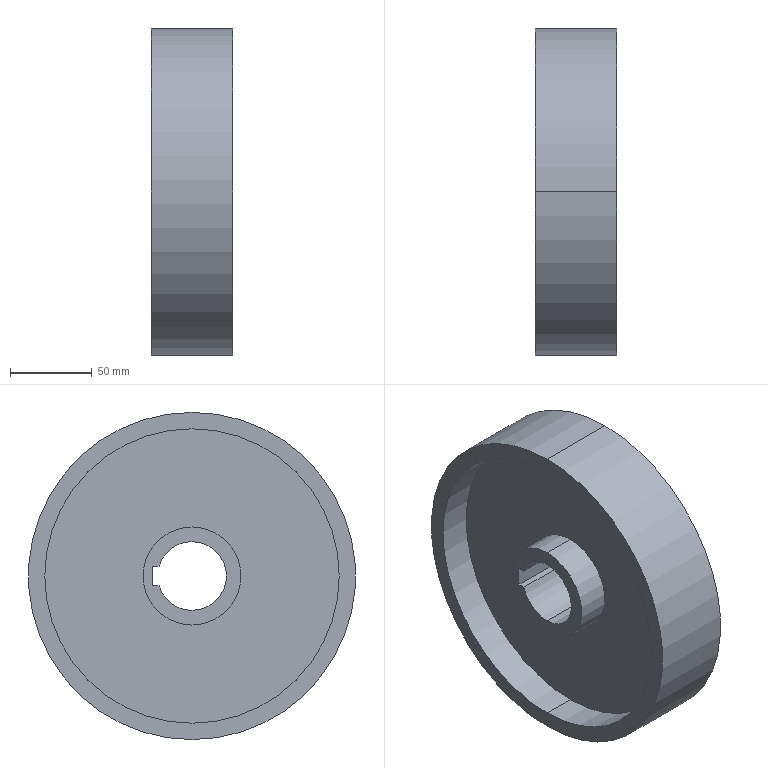Part | SolidWorks | features ICE 1, Revolution 1 | 1 solid | 22 faces | box 50 x 200 x 200 mm | volume 594592 mm3 | cylinder 13 | plane 9 | commonest cylinder face diameters 60 x4 180 x4 42 x3 200 x2
STEP:
#1=CARTESIAN_POINT('',(25.,0.,-21.));
#2=VERTEX_POINT('',#1);
#3=CARTESIAN_POINT('',(25.,0.,21.));
#4=VERTEX_POINT('',#3);
#5=CARTESIAN_POINT('',(25.,0.,0.));
#6=DIRECTION('',(-1.,0.,0.));
#7=DIRECTION('',(0.,0.,1.));
#8=AXIS2_PLACEMENT_3D('',#5,#6,#7);
#9=CIRCLE('',#8,21.);
#10=EDGE_CURVE('',#2,#4,#9,.T.);
#11=ORIENTED_EDGE('',*,*,#10,.F.);
#12=CARTESIAN_POINT('',(-25.,0.,-21.));
#13=VERTEX_POINT('',#12);
#14=CARTESIAN_POINT('',(0.,0.,-21.));
#15=DIRECTION('',(-1.,0.,0.));
#16=VECTOR('',#15,1000.);
#17=LINE('',#14,#16);
#18=EDGE_CURVE('',#2,#13,#17,.T.);
#19=ORIENTED_EDGE('',*,*,#18,.T.);
#20=CARTESIAN_POINT('',(-25.,0.,21.));
#21=VERTEX_POINT('',#20);
#22=CARTESIAN_POINT('',(-25.,0.,0.));
#23=DIRECTION('',(-1.,0.,0.));
#24=DIRECTION('',(0.,0.,1.));
#25=AXIS2_PLACEMENT_3D('',#22,#23,#24);
#26=CIRCLE('',#25,21.);
#27=EDGE_CURVE('',#13,#21,#26,.T.);
#28=ORIENTED_EDGE('',*,*,#27,.T.);
#29=CARTESIAN_POINT('',(0.,0.,21.));
#30=DIRECTION('',(-1.,0.,0.));
#31=VECTOR('',#30,1000.);
#32=LINE('',#29,#31);
#33=EDGE_CURVE('',#4,#21,#32,.T.);
#34=ORIENTED_EDGE('',*,*,#33,.F.);
#35=EDGE_LOOP('',(#11,#19,#28,#34));
#36=FACE_OUTER_BOUND('',#35,.T.);
#37=CARTESIAN_POINT('',(0.,0.,0.));
#38=DIRECTION('',(-1.,0.,0.));
#39=DIRECTION('',(0.,0.,1.));
#40=AXIS2_PLACEMENT_3D('',#37,#38,#39);
#41=CYLINDRICAL_SURFACE('',#40,21.);
#42=ADVANCED_FACE('',(#36),#41,.F.);
#43=CARTESIAN_POINT('',(25.,20.125,6.));
#44=VERTEX_POINT('',#43);
#45=CARTESIAN_POINT('',(25.,0.,0.));
#46=DIRECTION('',(-1.,0.,0.));
#47=DIRECTION('',(0.,0.,1.));
#48=AXIS2_PLACEMENT_3D('',#45,#46,#47);
#49=CIRCLE('',#48,21.);
#50=EDGE_CURVE('',#4,#44,#49,.T.);
#51=ORIENTED_EDGE('',*,*,#50,.F.);
#52=ORIENTED_EDGE('',*,*,#33,.T.);
#53=CARTESIAN_POINT('',(-25.,20.125,6.));
#54=VERTEX_POINT('',#53);
#55=CARTESIAN_POINT('',(-25.,0.,0.));
#56=DIRECTION('',(-1.,0.,0.));
#57=DIRECTION('',(0.,0.,1.));
#58=AXIS2_PLACEMENT_3D('',#55,#56,#57);
#59=CIRCLE('',#58,21.);
#60=EDGE_CURVE('',#21,#54,#59,.T.);
#61=ORIENTED_EDGE('',*,*,#60,.T.);
#62=CARTESIAN_POINT('',(0.,20.125,6.));
#63=DIRECTION('',(-1.,0.,0.));
#64=VECTOR('',#63,1000.);
#65=LINE('',#62,#64);
#66=EDGE_CURVE('',#44,#54,#65,.T.);
#67=ORIENTED_EDGE('',*,*,#66,.F.);
#68=EDGE_LOOP('',(#51,#52,#61,#67));
#69=FACE_OUTER_BOUND('',#68,.T.);
#70=CARTESIAN_POINT('',(0.,0.,0.));
#71=DIRECTION('',(-1.,0.,0.));
#72=DIRECTION('',(0.,0.,1.));
#73=AXIS2_PLACEMENT_3D('',#70,#71,#72);
#74=CYLINDRICAL_SURFACE('',#73,21.);
#75=ADVANCED_FACE('',(#69),#74,.F.);
#76=CARTESIAN_POINT('',(-5.,0.,30.));
#77=VERTEX_POINT('',#76);
#78=CARTESIAN_POINT('',(-5.,0.,-30.));
#79=VERTEX_POINT('',#78);
#80=CARTESIAN_POINT('',(-5.,0.,0.));
#81=DIRECTION('',(-1.,0.,0.));
#82=DIRECTION('',(0.,0.,1.));
#83=AXIS2_PLACEMENT_3D('',#80,#81,#82);
#84=CIRCLE('',#83,30.);
#85=EDGE_CURVE('',#77,#79,#84,.T.);
#86=ORIENTED_EDGE('',*,*,#85,.T.);
#87=CARTESIAN_POINT('',(-25.,0.,-30.));
#88=VERTEX_POINT('',#87);
#89=CARTESIAN_POINT('',(0.,0.,-30.));
#90=DIRECTION('',(-1.,0.,0.));
#91=VECTOR('',#90,1000.);
#92=LINE('',#89,#91);
#93=EDGE_CURVE('',#79,#88,#92,.T.);
#94=ORIENTED_EDGE('',*,*,#93,.T.);
#95=CARTESIAN_POINT('',(-25.,0.,30.));
#96=VERTEX_POINT('',#95);
#97=CARTESIAN_POINT('',(-25.,0.,0.));
#98=DIRECTION('',(-1.,0.,0.));
#99=DIRECTION('',(0.,0.,1.));
#100=AXIS2_PLACEMENT_3D('',#97,#98,#99);
#101=CIRCLE('',#100,30.);
#102=EDGE_CURVE('',#96,#88,#101,.T.);
#103=ORIENTED_EDGE('',*,*,#102,.F.);
#104=CARTESIAN_POINT('',(0.,0.,30.));
#105=DIRECTION('',(-1.,0.,0.));
#106=VECTOR('',#105,1000.);
#107=LINE('',#104,#106);
#108=EDGE_CURVE('',#77,#96,#107,.T.);
#109=ORIENTED_EDGE('',*,*,#108,.F.);
#110=EDGE_LOOP('',(#86,#94,#103,#109));
#111=FACE_OUTER_BOUND('',#110,.T.);
#112=CARTESIAN_POINT('',(0.,0.,0.));
#113=DIRECTION('',(-1.,0.,0.));
#114=DIRECTION('',(0.,0.,1.));
#115=AXIS2_PLACEMENT_3D('',#112,#113,#114);
#116=CYLINDRICAL_SURFACE('',#115,30.);
#117=ADVANCED_FACE('',(#111),#116,.T.);
#118=CARTESIAN_POINT('',(-5.,0.,-90.));
#119=VERTEX_POINT('',#118);
#120=CARTESIAN_POINT('',(-5.,0.,90.));
#121=VERTEX_POINT('',#120);
#122=CARTESIAN_POINT('',(-5.,0.,0.));
#123=DIRECTION('',(-1.,0.,0.));
#124=DIRECTION('',(0.,0.,1.));
#125=AXIS2_PLACEMENT_3D('',#122,#123,#124);
#126=CIRCLE('',#125,90.);
#127=EDGE_CURVE('',#119,#121,#126,.T.);
#128=ORIENTED_EDGE('',*,*,#127,.F.);
#129=CARTESIAN_POINT('',(-25.,0.,-90.));
#130=VERTEX_POINT('',#129);
#131=CARTESIAN_POINT('',(0.,0.,-90.));
#132=DIRECTION('',(-1.,0.,0.));
#133=VECTOR('',#132,1000.);
#134=LINE('',#131,#133);
#135=EDGE_CURVE('',#119,#130,#134,.T.);
#136=ORIENTED_EDGE('',*,*,#135,.T.);
#137=CARTESIAN_POINT('',(-25.,0.,90.));
#138=VERTEX_POINT('',#137);
#139=CARTESIAN_POINT('',(-25.,0.,0.));
#140=DIRECTION('',(-1.,0.,0.));
#141=DIRECTION('',(0.,0.,1.));
#142=AXIS2_PLACEMENT_3D('',#139,#140,#141);
#143=CIRCLE('',#142,90.);
#144=EDGE_CURVE('',#130,#138,#143,.T.);
#145=ORIENTED_EDGE('',*,*,#144,.T.);
#146=CARTESIAN_POINT('',(0.,0.,90.));
#147=DIRECTION('',(-1.,0.,0.));
#148=VECTOR('',#147,1000.);
#149=LINE('',#146,#148);
#150=EDGE_CURVE('',#121,#138,#149,.T.);
#151=ORIENTED_EDGE('',*,*,#150,.F.);
#152=EDGE_LOOP('',(#128,#136,#145,#151));
#153=FACE_OUTER_BOUND('',#152,.T.);
#154=CARTESIAN_POINT('',(0.,0.,0.));
#155=DIRECTION('',(-1.,0.,0.));
#156=DIRECTION('',(0.,0.,1.));
#157=AXIS2_PLACEMENT_3D('',#154,#155,#156);
#158=CYLINDRICAL_SURFACE('',#157,90.);
#159=ADVANCED_FACE('',(#153),#158,.F.);
#160=CARTESIAN_POINT('',(25.,0.,100.));
#161=VERTEX_POINT('',#160);
#162=CARTESIAN_POINT('',(25.,0.,-100.));
#163=VERTEX_POINT('',#162);
#164=CARTESIAN_POINT('',(25.,0.,0.));
#165=DIRECTION('',(-1.,0.,0.));
#166=DIRECTION('',(0.,0.,1.));
#167=AXIS2_PLACEMENT_3D('',#164,#165,#166);
#168=CIRCLE('',#167,100.);
#169=EDGE_CURVE('',#161,#163,#168,.T.);
#170=ORIENTED_EDGE('',*,*,#169,.T.);
#171=CARTESIAN_POINT('',(-25.,0.,-100.));
#172=VERTEX_POINT('',#171);
#173=CARTESIAN_POINT('',(0.,0.,-100.));
#174=DIRECTION('',(-1.,0.,0.));
#175=VECTOR('',#174,1000.);
#176=LINE('',#173,#175);
#177=EDGE_CURVE('',#163,#172,#176,.T.);
#178=ORIENTED_EDGE('',*,*,#177,.T.);
#179=CARTESIAN_POINT('',(-25.,0.,100.));
#180=VERTEX_POINT('',#179);
#181=CARTESIAN_POINT('',(-25.,0.,0.));
#182=DIRECTION('',(-1.,0.,0.));
#183=DIRECTION('',(0.,0.,1.));
#184=AXIS2_PLACEMENT_3D('',#181,#182,#183);
#185=CIRCLE('',#184,100.);
#186=EDGE_CURVE('',#180,#172,#185,.T.);
#187=ORIENTED_EDGE('',*,*,#186,.F.);
#188=CARTESIAN_POINT('',(0.,0.,100.));
#189=DIRECTION('',(-1.,0.,0.));
#190=VECTOR('',#189,1000.);
#191=LINE('',#188,#190);
#192=EDGE_CURVE('',#161,#180,#191,.T.);
#193=ORIENTED_EDGE('',*,*,#192,.F.);
#194=EDGE_LOOP('',(#170,#178,#187,#193));
#195=FACE_OUTER_BOUND('',#194,.T.);
#196=CARTESIAN_POINT('',(0.,0.,0.));
#197=DIRECTION('',(-1.,0.,0.));
#198=DIRECTION('',(0.,0.,1.));
#199=AXIS2_PLACEMENT_3D('',#196,#197,#198);
#200=CYLINDRICAL_SURFACE('',#199,100.);
#201=ADVANCED_FACE('',(#195),#200,.T.);
#202=CARTESIAN_POINT('',(25.,0.,-90.));
#203=VERTEX_POINT('',#202);
#204=CARTESIAN_POINT('',(25.,0.,90.));
#205=VERTEX_POINT('',#204);
#206=CARTESIAN_POINT('',(25.,0.,0.));
#207=DIRECTION('',(-1.,0.,0.));
#208=DIRECTION('',(0.,0.,1.));
#209=AXIS2_PLACEMENT_3D('',#206,#207,#208);
#210=CIRCLE('',#209,90.);
#211=EDGE_CURVE('',#203,#205,#210,.T.);
#212=ORIENTED_EDGE('',*,*,#211,.F.);
#213=CARTESIAN_POINT('',(5.,0.,-90.));
#214=VERTEX_POINT('',#213);
#215=CARTESIAN_POINT('',(0.,0.,-90.));
#216=DIRECTION('',(-1.,0.,0.));
#217=VECTOR('',#216,1000.);
#218=LINE('',#215,#217);
#219=EDGE_CURVE('',#203,#214,#218,.T.);
#220=ORIENTED_EDGE('',*,*,#219,.T.);
#221=CARTESIAN_POINT('',(5.,0.,90.));
#222=VERTEX_POINT('',#221);
#223=CARTESIAN_POINT('',(5.,0.,0.));
#224=DIRECTION('',(-1.,0.,0.));
#225=DIRECTION('',(0.,0.,1.));
#226=AXIS2_PLACEMENT_3D('',#223,#224,#225);
#227=CIRCLE('',#226,90.);
#228=EDGE_CURVE('',#214,#222,#227,.T.);
#229=ORIENTED_EDGE('',*,*,#228,.T.);
#230=CARTESIAN_POINT('',(0.,0.,90.));
#231=DIRECTION('',(-1.,0.,0.));
#232=VECTOR('',#231,1000.);
#233=LINE('',#230,#232);
#234=EDGE_CURVE('',#205,#222,#233,.T.);
#235=ORIENTED_EDGE('',*,*,#234,.F.);
#236=EDGE_LOOP('',(#212,#220,#229,#235));
#237=FACE_OUTER_BOUND('',#236,.T.);
#238=CARTESIAN_POINT('',(0.,0.,0.));
#239=DIRECTION('',(-1.,0.,0.));
#240=DIRECTION('',(0.,0.,1.));
#241=AXIS2_PLACEMENT_3D('',#238,#239,#240);
#242=CYLINDRICAL_SURFACE('',#241,90.);
#243=ADVANCED_FACE('',(#237),#242,.F.);
#244=CARTESIAN_POINT('',(25.,0.,30.));
#245=VERTEX_POINT('',#244);
#246=CARTESIAN_POINT('',(25.,0.,-30.));
#247=VERTEX_POINT('',#246);
#248=CARTESIAN_POINT('',(25.,0.,0.));
#249=DIRECTION('',(-1.,0.,0.));
#250=DIRECTION('',(0.,0.,1.));
#251=AXIS2_PLACEMENT_3D('',#248,#249,#250);
#252=CIRCLE('',#251,30.);
#253=EDGE_CURVE('',#245,#247,#252,.T.);
#254=ORIENTED_EDGE('',*,*,#253,.T.);
#255=CARTESIAN_POINT('',(5.,0.,-30.));
#256=VERTEX_POINT('',#255);
#257=CARTESIAN_POINT('',(0.,0.,-30.));
#258=DIRECTION('',(-1.,0.,0.));
#259=VECTOR('',#258,1000.);
#260=LINE('',#257,#259);
#261=EDGE_CURVE('',#247,#256,#260,.T.);
#262=ORIENTED_EDGE('',*,*,#261,.T.);
#263=CARTESIAN_POINT('',(5.,0.,30.));
#264=VERTEX_POINT('',#263);
#265=CARTESIAN_POINT('',(5.,0.,0.));
#266=DIRECTION('',(-1.,0.,0.));
#267=DIRECTION('',(0.,0.,1.));
#268=AXIS2_PLACEMENT_3D('',#265,#266,#267);
#269=CIRCLE('',#268,30.);
#270=EDGE_CURVE('',#264,#256,#269,.T.);
#271=ORIENTED_EDGE('',*,*,#270,.F.);
#272=CARTESIAN_POINT('',(0.,0.,30.));
#273=DIRECTION('',(-1.,0.,0.));
#274=VECTOR('',#273,1000.);
#275=LINE('',#272,#274);
#276=EDGE_CURVE('',#245,#264,#275,.T.);
#277=ORIENTED_EDGE('',*,*,#276,.F.);
#278=EDGE_LOOP('',(#254,#262,#271,#277));
#279=FACE_OUTER_BOUND('',#278,.T.);
#280=CARTESIAN_POINT('',(0.,0.,0.));
#281=DIRECTION('',(-1.,0.,0.));
#282=DIRECTION('',(0.,0.,1.));
#283=AXIS2_PLACEMENT_3D('',#280,#281,#282);
#284=CYLINDRICAL_SURFACE('',#283,30.);
#285=ADVANCED_FACE('',(#279),#284,.T.);
#286=ORIENTED_EDGE('',*,*,#253,.F.);
#287=CARTESIAN_POINT('',(25.,0.,0.));
#288=DIRECTION('',(-1.,0.,0.));
#289=DIRECTION('',(0.,0.,1.));
#290=AXIS2_PLACEMENT_3D('',#287,#288,#289);
#291=CIRCLE('',#290,30.);
#292=EDGE_CURVE('',#247,#245,#291,.T.);
#293=ORIENTED_EDGE('',*,*,#292,.F.);
#294=EDGE_LOOP('',(#286,#293));
#295=FACE_OUTER_BOUND('',#294,.T.);
#296=CARTESIAN_POINT('',(25.,20.125,-6.));
#297=VERTEX_POINT('',#296);
#298=CARTESIAN_POINT('',(25.,0.,0.));
#299=DIRECTION('',(-1.,0.,0.));
#300=DIRECTION('',(0.,0.,1.));
#301=AXIS2_PLACEMENT_3D('',#298,#299,#300);
#302=CIRCLE('',#301,21.);
#303=EDGE_CURVE('',#297,#2,#302,.T.);
#304=ORIENTED_EDGE('',*,*,#303,.T.);
#305=ORIENTED_EDGE('',*,*,#10,.T.);
#306=ORIENTED_EDGE('',*,*,#50,.T.);
#307=CARTESIAN_POINT('',(25.,24.3,6.));
#308=VERTEX_POINT('',#307);
#309=CARTESIAN_POINT('',(25.,17.7,6.));
#310=DIRECTION('',(0.,-1.,0.));
#311=VECTOR('',#310,1000.);
#312=LINE('',#309,#311);
#313=EDGE_CURVE('',#308,#44,#312,.T.);
#314=ORIENTED_EDGE('',*,*,#313,.F.);
#315=CARTESIAN_POINT('',(25.,24.3,-6.));
#316=VERTEX_POINT('',#315);
#317=CARTESIAN_POINT('',(25.,24.3,-6.));
#318=DIRECTION('',(0.,0.,1.));
#319=VECTOR('',#318,1000.);
#320=LINE('',#317,#319);
#321=EDGE_CURVE('',#316,#308,#320,.T.);
#322=ORIENTED_EDGE('',*,*,#321,.F.);
#323=CARTESIAN_POINT('',(25.,17.7,-6.));
#324=DIRECTION('',(0.,1.,0.));
#325=VECTOR('',#324,1000.);
#326=LINE('',#323,#325);
#327=EDGE_CURVE('',#297,#316,#326,.T.);
#328=ORIENTED_EDGE('',*,*,#327,.F.);
#329=EDGE_LOOP('',(#304,#305,#306,#314,#322,#328));
#330=FACE_BOUND('',#329,.T.);
#331=CARTESIAN_POINT('',(25.,21.,0.));
#332=DIRECTION('',(-1.,0.,0.));
#333=DIRECTION('',(0.,0.,1.));
#334=AXIS2_PLACEMENT_3D('',#331,#332,#333);
#335=PLANE('',#334);
#336=ADVANCED_FACE('',(#295,#330),#335,.F.);
#337=ORIENTED_EDGE('',*,*,#261,.F.);
#338=ORIENTED_EDGE('',*,*,#292,.T.);
#339=ORIENTED_EDGE('',*,*,#276,.T.);
#340=CARTESIAN_POINT('',(5.,0.,0.));
#341=DIRECTION('',(-1.,0.,0.));
#342=DIRECTION('',(0.,0.,1.));
#343=AXIS2_PLACEMENT_3D('',#340,#341,#342);
#344=CIRCLE('',#343,30.);
#345=EDGE_CURVE('',#256,#264,#344,.T.);
#346=ORIENTED_EDGE('',*,*,#345,.F.);
#347=EDGE_LOOP('',(#337,#338,#339,#346));
#348=FACE_OUTER_BOUND('',#347,.T.);
#349=CARTESIAN_POINT('',(0.,0.,0.));
#350=DIRECTION('',(-1.,0.,0.));
#351=DIRECTION('',(0.,0.,1.));
#352=AXIS2_PLACEMENT_3D('',#349,#350,#351);
#353=CYLINDRICAL_SURFACE('',#352,30.);
#354=ADVANCED_FACE('',(#348),#353,.T.);
#355=CARTESIAN_POINT('',(5.,0.,0.));
#356=DIRECTION('',(-1.,0.,0.));
#357=DIRECTION('',(0.,0.,1.));
#358=AXIS2_PLACEMENT_3D('',#355,#356,#357);
#359=CIRCLE('',#358,90.);
#360=EDGE_CURVE('',#222,#214,#359,.T.);
#361=ORIENTED_EDGE('',*,*,#360,.F.);
#362=ORIENTED_EDGE('',*,*,#228,.F.);
#363=EDGE_LOOP('',(#361,#362));
#364=FACE_OUTER_BOUND('',#363,.T.);
#365=ORIENTED_EDGE('',*,*,#270,.T.);
#366=ORIENTED_EDGE('',*,*,#345,.T.);
#367=EDGE_LOOP('',(#365,#366));
#368=FACE_BOUND('',#367,.T.);
#369=CARTESIAN_POINT('',(5.,30.,0.));
#370=DIRECTION('',(-1.,0.,0.));
#371=DIRECTION('',(0.,0.,1.));
#372=AXIS2_PLACEMENT_3D('',#369,#370,#371);
#373=PLANE('',#372);
#374=ADVANCED_FACE('',(#364,#368),#373,.F.);
#375=ORIENTED_EDGE('',*,*,#219,.F.);
#376=CARTESIAN_POINT('',(25.,0.,0.));
#377=DIRECTION('',(-1.,0.,0.));
#378=DIRECTION('',(0.,0.,1.));
#379=AXIS2_PLACEMENT_3D('',#376,#377,#378);
#380=CIRCLE('',#379,90.);
#381=EDGE_CURVE('',#205,#203,#380,.T.);
#382=ORIENTED_EDGE('',*,*,#381,.F.);
#383=ORIENTED_EDGE('',*,*,#234,.T.);
#384=ORIENTED_EDGE('',*,*,#360,.T.);
#385=EDGE_LOOP('',(#375,#382,#383,#384));
#386=FACE_OUTER_BOUND('',#385,.T.);
#387=CARTESIAN_POINT('',(0.,0.,0.));
#388=DIRECTION('',(-1.,0.,0.));
#389=DIRECTION('',(0.,0.,1.));
#390=AXIS2_PLACEMENT_3D('',#387,#388,#389);
#391=CYLINDRICAL_SURFACE('',#390,90.);
#392=ADVANCED_FACE('',(#386),#391,.F.);
#393=ORIENTED_EDGE('',*,*,#169,.F.);
#394=CARTESIAN_POINT('',(25.,0.,0.));
#395=DIRECTION('',(-1.,0.,0.));
#396=DIRECTION('',(0.,0.,1.));
#397=AXIS2_PLACEMENT_3D('',#394,#395,#396);
#398=CIRCLE('',#397,100.);
#399=EDGE_CURVE('',#163,#161,#398,.T.);
#400=ORIENTED_EDGE('',*,*,#399,.F.);
#401=EDGE_LOOP('',(#393,#400));
#402=FACE_OUTER_BOUND('',#401,.T.);
#403=ORIENTED_EDGE('',*,*,#381,.T.);
#404=ORIENTED_EDGE('',*,*,#211,.T.);
#405=EDGE_LOOP('',(#403,#404));
#406=FACE_BOUND('',#405,.T.);
#407=CARTESIAN_POINT('',(25.,90.,0.));
#408=DIRECTION('',(-1.,0.,0.));
#409=DIRECTION('',(0.,0.,1.));
#410=AXIS2_PLACEMENT_3D('',#407,#408,#409);
#411=PLANE('',#410);
#412=ADVANCED_FACE('',(#402,#406),#411,.F.);
#413=ORIENTED_EDGE('',*,*,#177,.F.);
#414=ORIENTED_EDGE('',*,*,#399,.T.);
#415=ORIENTED_EDGE('',*,*,#192,.T.);
#416=CARTESIAN_POINT('',(-25.,0.,0.));
#417=DIRECTION('',(-1.,0.,0.));
#418=DIRECTION('',(0.,0.,1.));
#419=AXIS2_PLACEMENT_3D('',#416,#417,#418);
#420=CIRCLE('',#419,100.);
#421=EDGE_CURVE('',#172,#180,#420,.T.);
#422=ORIENTED_EDGE('',*,*,#421,.F.);
#423=EDGE_LOOP('',(#413,#414,#415,#422));
#424=FACE_OUTER_BOUND('',#423,.T.);
#425=CARTESIAN_POINT('',(0.,0.,0.));
#426=DIRECTION('',(-1.,0.,0.));
#427=DIRECTION('',(0.,0.,1.));
#428=AXIS2_PLACEMENT_3D('',#425,#426,#427);
#429=CYLINDRICAL_SURFACE('',#428,100.);
#430=ADVANCED_FACE('',(#424),#429,.T.);
#431=CARTESIAN_POINT('',(-25.,0.,0.));
#432=DIRECTION('',(-1.,0.,0.));
#433=DIRECTION('',(0.,0.,1.));
#434=AXIS2_PLACEMENT_3D('',#431,#432,#433);
#435=CIRCLE('',#434,90.);
#436=EDGE_CURVE('',#138,#130,#435,.T.);
#437=ORIENTED_EDGE('',*,*,#436,.F.);
#438=ORIENTED_EDGE('',*,*,#144,.F.);
#439=EDGE_LOOP('',(#437,#438));
#440=FACE_BOUND('',#439,.T.);
#441=ORIENTED_EDGE('',*,*,#186,.T.);
#442=ORIENTED_EDGE('',*,*,#421,.T.);
#443=EDGE_LOOP('',(#441,#442));
#444=FACE_OUTER_BOUND('',#443,.T.);
#445=CARTESIAN_POINT('',(-25.,90.,0.));
#446=DIRECTION('',(1.,0.,0.));
#447=DIRECTION('',(0.,0.,-1.));
#448=AXIS2_PLACEMENT_3D('',#445,#446,#447);
#449=PLANE('',#448);
#450=ADVANCED_FACE('',(#440,#444),#449,.F.);
#451=ORIENTED_EDGE('',*,*,#135,.F.);
#452=CARTESIAN_POINT('',(-5.,0.,0.));
#453=DIRECTION('',(-1.,0.,0.));
#454=DIRECTION('',(0.,0.,1.));
#455=AXIS2_PLACEMENT_3D('',#452,#453,#454);
#456=CIRCLE('',#455,90.);
#457=EDGE_CURVE('',#121,#119,#456,.T.);
#458=ORIENTED_EDGE('',*,*,#457,.F.);
#459=ORIENTED_EDGE('',*,*,#150,.T.);
#460=ORIENTED_EDGE('',*,*,#436,.T.);
#461=EDGE_LOOP('',(#451,#458,#459,#460));
#462=FACE_OUTER_BOUND('',#461,.T.);
#463=CARTESIAN_POINT('',(0.,0.,0.));
#464=DIRECTION('',(-1.,0.,0.));
#465=DIRECTION('',(0.,0.,1.));
#466=AXIS2_PLACEMENT_3D('',#463,#464,#465);
#467=CYLINDRICAL_SURFACE('',#466,90.);
#468=ADVANCED_FACE('',(#462),#467,.F.);
#469=ORIENTED_EDGE('',*,*,#85,.F.);
#470=CARTESIAN_POINT('',(-5.,0.,0.));
#471=DIRECTION('',(-1.,0.,0.));
#472=DIRECTION('',(0.,0.,1.));
#473=AXIS2_PLACEMENT_3D('',#470,#471,#472);
#474=CIRCLE('',#473,30.);
#475=EDGE_CURVE('',#79,#77,#474,.T.);
#476=ORIENTED_EDGE('',*,*,#475,.F.);
#477=EDGE_LOOP('',(#469,#476));
#478=FACE_BOUND('',#477,.T.);
#479=ORIENTED_EDGE('',*,*,#457,.T.);
#480=ORIENTED_EDGE('',*,*,#127,.T.);
#481=EDGE_LOOP('',(#479,#480));
#482=FACE_OUTER_BOUND('',#481,.T.);
#483=CARTESIAN_POINT('',(-5.,30.,0.));
#484=DIRECTION('',(1.,0.,0.));
#485=DIRECTION('',(0.,0.,-1.));
#486=AXIS2_PLACEMENT_3D('',#483,#484,#485);
#487=PLANE('',#486);
#488=ADVANCED_FACE('',(#478,#482),#487,.F.);
#489=ORIENTED_EDGE('',*,*,#93,.F.);
#490=ORIENTED_EDGE('',*,*,#475,.T.);
#491=ORIENTED_EDGE('',*,*,#108,.T.);
#492=CARTESIAN_POINT('',(-25.,0.,0.));
#493=DIRECTION('',(-1.,0.,0.));
#494=DIRECTION('',(0.,0.,1.));
#495=AXIS2_PLACEMENT_3D('',#492,#493,#494);
#496=CIRCLE('',#495,30.);
#497=EDGE_CURVE('',#88,#96,#496,.T.);
#498=ORIENTED_EDGE('',*,*,#497,.F.);
#499=EDGE_LOOP('',(#489,#490,#491,#498));
#500=FACE_OUTER_BOUND('',#499,.T.);
#501=CARTESIAN_POINT('',(0.,0.,0.));
#502=DIRECTION('',(-1.,0.,0.));
#503=DIRECTION('',(0.,0.,1.));
#504=AXIS2_PLACEMENT_3D('',#501,#502,#503);
#505=CYLINDRICAL_SURFACE('',#504,30.);
#506=ADVANCED_FACE('',(#500),#505,.T.);
#507=CARTESIAN_POINT('',(-25.,24.3,6.));
#508=VERTEX_POINT('',#507);
#509=CARTESIAN_POINT('',(-25.,24.3,-6.));
#510=VERTEX_POINT('',#509);
#511=CARTESIAN_POINT('',(-25.,24.3,-6.));
#512=DIRECTION('',(0.,0.,-1.));
#513=VECTOR('',#512,1000.);
#514=LINE('',#511,#513);
#515=EDGE_CURVE('',#508,#510,#514,.T.);
#516=ORIENTED_EDGE('',*,*,#515,.F.);
#517=CARTESIAN_POINT('',(-25.,17.7,6.));
#518=DIRECTION('',(0.,1.,0.));
#519=VECTOR('',#518,1000.);
#520=LINE('',#517,#519);
#521=EDGE_CURVE('',#54,#508,#520,.T.);
#522=ORIENTED_EDGE('',*,*,#521,.F.);
#523=ORIENTED_EDGE('',*,*,#60,.F.);
#524=ORIENTED_EDGE('',*,*,#27,.F.);
#525=CARTESIAN_POINT('',(-25.,20.125,-6.));
#526=VERTEX_POINT('',#525);
#527=CARTESIAN_POINT('',(-25.,0.,0.));
#528=DIRECTION('',(-1.,0.,0.));
#529=DIRECTION('',(0.,0.,1.));
#530=AXIS2_PLACEMENT_3D('',#527,#528,#529);
#531=CIRCLE('',#530,21.);
#532=EDGE_CURVE('',#526,#13,#531,.T.);
#533=ORIENTED_EDGE('',*,*,#532,.F.);
#534=CARTESIAN_POINT('',(-25.,17.7,-6.));
#535=DIRECTION('',(0.,-1.,0.));
#536=VECTOR('',#535,1000.);
#537=LINE('',#534,#536);
#538=EDGE_CURVE('',#510,#526,#537,.T.);
#539=ORIENTED_EDGE('',*,*,#538,.F.);
#540=EDGE_LOOP('',(#516,#522,#523,#524,#533,#539));
#541=FACE_BOUND('',#540,.T.);
#542=ORIENTED_EDGE('',*,*,#102,.T.);
#543=ORIENTED_EDGE('',*,*,#497,.T.);
#544=EDGE_LOOP('',(#542,#543));
#545=FACE_OUTER_BOUND('',#544,.T.);
#546=CARTESIAN_POINT('',(-25.,21.,0.));
#547=DIRECTION('',(1.,0.,0.));
#548=DIRECTION('',(0.,0.,-1.));
#549=AXIS2_PLACEMENT_3D('',#546,#547,#548);
#550=PLANE('',#549);
#551=ADVANCED_FACE('',(#541,#545),#550,.F.);
#552=ORIENTED_EDGE('',*,*,#18,.F.);
#553=ORIENTED_EDGE('',*,*,#303,.F.);
#554=CARTESIAN_POINT('',(0.,20.125,-6.));
#555=DIRECTION('',(1.,0.,0.));
#556=VECTOR('',#555,1000.);
#557=LINE('',#554,#556);
#558=EDGE_CURVE('',#526,#297,#557,.T.);
#559=ORIENTED_EDGE('',*,*,#558,.F.);
#560=ORIENTED_EDGE('',*,*,#532,.T.);
#561=EDGE_LOOP('',(#552,#553,#559,#560));
#562=FACE_OUTER_BOUND('',#561,.T.);
#563=CARTESIAN_POINT('',(0.,0.,0.));
#564=DIRECTION('',(-1.,0.,0.));
#565=DIRECTION('',(0.,0.,1.));
#566=AXIS2_PLACEMENT_3D('',#563,#564,#565);
#567=CYLINDRICAL_SURFACE('',#566,21.);
#568=ADVANCED_FACE('',(#562),#567,.F.);
#569=ORIENTED_EDGE('',*,*,#521,.T.);
#570=CARTESIAN_POINT('',(-25.001,24.3,6.));
#571=DIRECTION('',(1.,0.,0.));
#572=VECTOR('',#571,1000.);
#573=LINE('',#570,#572);
#574=EDGE_CURVE('',#508,#308,#573,.T.);
#575=ORIENTED_EDGE('',*,*,#574,.T.);
#576=ORIENTED_EDGE('',*,*,#313,.T.);
#577=ORIENTED_EDGE('',*,*,#66,.T.);
#578=EDGE_LOOP('',(#569,#575,#576,#577));
#579=FACE_OUTER_BOUND('',#578,.T.);
#580=CARTESIAN_POINT('',(-25.001,17.7,6.));
#581=DIRECTION('',(0.,0.,1.));
#582=DIRECTION('',(1.,0.,0.));
#583=AXIS2_PLACEMENT_3D('',#580,#581,#582);
#584=PLANE('',#583);
#585=ADVANCED_FACE('',(#579),#584,.F.);
#586=ORIENTED_EDGE('',*,*,#515,.T.);
#587=CARTESIAN_POINT('',(-25.001,24.3,-6.));
#588=DIRECTION('',(1.,0.,0.));
#589=VECTOR('',#588,1000.);
#590=LINE('',#587,#589);
#591=EDGE_CURVE('',#510,#316,#590,.T.);
#592=ORIENTED_EDGE('',*,*,#591,.T.);
#593=ORIENTED_EDGE('',*,*,#321,.T.);
#594=ORIENTED_EDGE('',*,*,#574,.F.);
#595=EDGE_LOOP('',(#586,#592,#593,#594));
#596=FACE_OUTER_BOUND('',#595,.T.);
#597=CARTESIAN_POINT('',(-25.001,24.3,-6.));
#598=DIRECTION('',(0.,1.,0.));
#599=DIRECTION('',(0.,0.,1.));
#600=AXIS2_PLACEMENT_3D('',#597,#598,#599);
#601=PLANE('',#600);
#602=ADVANCED_FACE('',(#596),#601,.F.);
#603=ORIENTED_EDGE('',*,*,#538,.T.);
#604=ORIENTED_EDGE('',*,*,#558,.T.);
#605=ORIENTED_EDGE('',*,*,#327,.T.);
#606=ORIENTED_EDGE('',*,*,#591,.F.);
#607=EDGE_LOOP('',(#603,#604,#605,#606));
#608=FACE_OUTER_BOUND('',#607,.T.);
#609=CARTESIAN_POINT('',(-25.001,17.7,-6.));
#610=DIRECTION('',(0.,0.,-1.));
#611=DIRECTION('',(-1.,0.,0.));
#612=AXIS2_PLACEMENT_3D('',#609,#610,#611);
#613=PLANE('',#612);
#614=ADVANCED_FACE('',(#608),#613,.F.);
#615=CLOSED_SHELL('',(#42,#75,#117,#159,#201,#243,#285,#336,#354,#374,#392,#412,#430,#450,#468,#488,#506,#551,#568,#585,#602,#614));
#616=MANIFOLD_SOLID_BREP('',#615);
#617=CARTESIAN_POINT('',(0.,0.,0.));
#618=DIRECTION('',(0.,0.,1.));
#619=DIRECTION('',(1.,0.,0.));
#620=AXIS2_PLACEMENT_3D('',#617,#618,#619);
#621=(LENGTH_UNIT()NAMED_UNIT(*)SI_UNIT(.MILLI.,.METRE.));
#622=UNCERTAINTY_MEASURE_WITH_UNIT(LENGTH_MEASURE(0.00001),#621,'','');
#623=(NAMED_UNIT(*)PLANE_ANGLE_UNIT()SI_UNIT($,.RADIAN.));
#624=(NAMED_UNIT(*)SI_UNIT($,.STERADIAN.)SOLID_ANGLE_UNIT());
#625=(GEOMETRIC_REPRESENTATION_CONTEXT(3)GLOBAL_UNCERTAINTY_ASSIGNED_CONTEXT((#622))GLOBAL_UNIT_ASSIGNED_CONTEXT((#621,#623,#624))REPRESENTATION_CONTEXT('',''));
#626=ADVANCED_BREP_SHAPE_REPRESENTATION('',(#616,#620),#625);